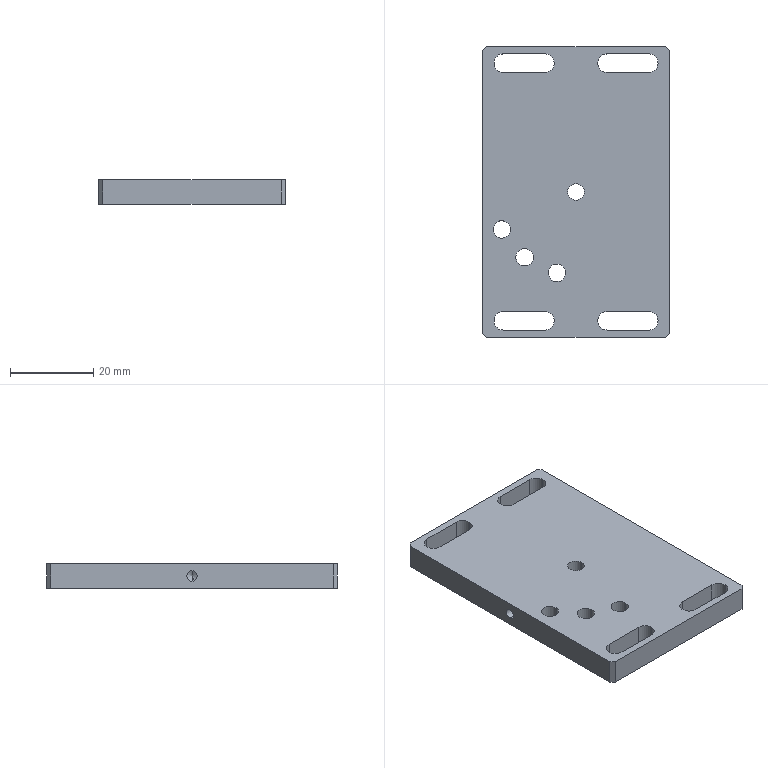Part | NX | features BREP 1 | 1 solid | 46 faces | box 45 x 70 x 6 mm | volume 16957 mm3 | cylinder 24 | plane 18 | cone 4 | commonest cylinder face diameters 4.5 x12 4.2 x6 2.5 x4 4 x2
STEP:
#1=CARTESIAN_POINT('',(2.,0.,6.));
#2=VERTEX_POINT('',#1);
#3=CARTESIAN_POINT('',(-2.,0.,6.));
#4=VERTEX_POINT('',#3);
#5=CARTESIAN_POINT('',(0.,0.,6.));
#6=DIRECTION('',(0.,0.,-1.));
#7=DIRECTION('',(-1.,0.,0.));
#8=AXIS2_PLACEMENT_3D('',#5,#6,#7);
#9=CIRCLE('',#8,2.);
#10=EDGE_CURVE('',#2,#4,#9,.T.);
#11=ORIENTED_EDGE('',*,*,#10,.F.);
#12=CARTESIAN_POINT('',(2.,0.,0.));
#13=VERTEX_POINT('',#12);
#14=CARTESIAN_POINT('',(2.,0.,0.));
#15=DIRECTION('',(0.,0.,-1.));
#16=VECTOR('',#15,1000.);
#17=LINE('',#14,#16);
#18=EDGE_CURVE('',#2,#13,#17,.T.);
#19=ORIENTED_EDGE('',*,*,#18,.T.);
#20=CARTESIAN_POINT('',(-2.,0.,0.));
#21=VERTEX_POINT('',#20);
#22=CARTESIAN_POINT('',(0.,0.,0.));
#23=DIRECTION('',(0.,0.,-1.));
#24=DIRECTION('',(-1.,0.,0.));
#25=AXIS2_PLACEMENT_3D('',#22,#23,#24);
#26=CIRCLE('',#25,2.);
#27=EDGE_CURVE('',#13,#21,#26,.T.);
#28=ORIENTED_EDGE('',*,*,#27,.T.);
#29=CARTESIAN_POINT('',(-2.,0.,0.));
#30=DIRECTION('',(0.,0.,-1.));
#31=VECTOR('',#30,1000.);
#32=LINE('',#29,#31);
#33=EDGE_CURVE('',#4,#21,#32,.T.);
#34=ORIENTED_EDGE('',*,*,#33,.F.);
#35=EDGE_LOOP('',(#11,#19,#28,#34));
#36=FACE_BOUND('',#35,.T.);
#37=CARTESIAN_POINT('',(0.,0.,0.));
#38=DIRECTION('',(0.,0.,-1.));
#39=DIRECTION('',(-1.,0.,0.));
#40=AXIS2_PLACEMENT_3D('',#37,#38,#39);
#41=CYLINDRICAL_SURFACE('',#40,2.);
#42=ADVANCED_FACE('',(#36),#41,.F.);
#43=CARTESIAN_POINT('',(-6.686,-19.467,0.));
#44=VERTEX_POINT('',#43);
#45=CARTESIAN_POINT('',(-2.486,-19.467,0.));
#46=VERTEX_POINT('',#45);
#47=CARTESIAN_POINT('',(-4.586,-19.467,0.));
#48=DIRECTION('',(0.,0.,1.));
#49=DIRECTION('',(1.,0.,0.));
#50=AXIS2_PLACEMENT_3D('',#47,#48,#49);
#51=CIRCLE('',#50,2.1);
#52=EDGE_CURVE('',#44,#46,#51,.T.);
#53=ORIENTED_EDGE('',*,*,#52,.F.);
#54=CARTESIAN_POINT('',(-6.686,-19.467,6.));
#55=VERTEX_POINT('',#54);
#56=CARTESIAN_POINT('',(-6.686,-19.467,6.));
#57=DIRECTION('',(0.,0.,1.));
#58=VECTOR('',#57,1000.);
#59=LINE('',#56,#58);
#60=EDGE_CURVE('',#55,#44,#59,.F.);
#61=ORIENTED_EDGE('',*,*,#60,.F.);
#62=CARTESIAN_POINT('',(-2.486,-19.467,6.));
#63=VERTEX_POINT('',#62);
#64=CARTESIAN_POINT('',(-4.586,-19.467,6.));
#65=DIRECTION('',(0.,0.,1.));
#66=DIRECTION('',(1.,0.,0.));
#67=AXIS2_PLACEMENT_3D('',#64,#65,#66);
#68=CIRCLE('',#67,2.1);
#69=EDGE_CURVE('',#55,#63,#68,.T.);
#70=ORIENTED_EDGE('',*,*,#69,.T.);
#71=CARTESIAN_POINT('',(-2.486,-19.467,6.));
#72=DIRECTION('',(0.,0.,1.));
#73=VECTOR('',#72,1000.);
#74=LINE('',#71,#73);
#75=EDGE_CURVE('',#63,#46,#74,.F.);
#76=ORIENTED_EDGE('',*,*,#75,.T.);
#77=EDGE_LOOP('',(#53,#61,#70,#76));
#78=FACE_BOUND('',#77,.T.);
#79=CARTESIAN_POINT('',(-4.586,-19.467,6.));
#80=DIRECTION('',(0.,0.,1.));
#81=DIRECTION('',(1.,0.,0.));
#82=AXIS2_PLACEMENT_3D('',#79,#80,#81);
#83=CYLINDRICAL_SURFACE('',#82,2.1);
#84=ADVANCED_FACE('',(#78),#83,.F.);
#85=CARTESIAN_POINT('',(-14.484,-15.705,0.));
#86=VERTEX_POINT('',#85);
#87=CARTESIAN_POINT('',(-10.284,-15.705,0.));
#88=VERTEX_POINT('',#87);
#89=CARTESIAN_POINT('',(-12.384,-15.705,0.));
#90=DIRECTION('',(0.,0.,1.));
#91=DIRECTION('',(1.,0.,0.));
#92=AXIS2_PLACEMENT_3D('',#89,#90,#91);
#93=CIRCLE('',#92,2.1);
#94=EDGE_CURVE('',#86,#88,#93,.T.);
#95=ORIENTED_EDGE('',*,*,#94,.F.);
#96=CARTESIAN_POINT('',(-14.484,-15.705,6.));
#97=VERTEX_POINT('',#96);
#98=CARTESIAN_POINT('',(-14.484,-15.705,6.));
#99=DIRECTION('',(0.,0.,1.));
#100=VECTOR('',#99,1000.);
#101=LINE('',#98,#100);
#102=EDGE_CURVE('',#97,#86,#101,.F.);
#103=ORIENTED_EDGE('',*,*,#102,.F.);
#104=CARTESIAN_POINT('',(-10.284,-15.705,6.));
#105=VERTEX_POINT('',#104);
#106=CARTESIAN_POINT('',(-12.384,-15.705,6.));
#107=DIRECTION('',(0.,0.,1.));
#108=DIRECTION('',(1.,0.,0.));
#109=AXIS2_PLACEMENT_3D('',#106,#107,#108);
#110=CIRCLE('',#109,2.1);
#111=EDGE_CURVE('',#97,#105,#110,.T.);
#112=ORIENTED_EDGE('',*,*,#111,.T.);
#113=CARTESIAN_POINT('',(-10.284,-15.705,6.));
#114=DIRECTION('',(0.,0.,1.));
#115=VECTOR('',#114,1000.);
#116=LINE('',#113,#115);
#117=EDGE_CURVE('',#105,#88,#116,.F.);
#118=ORIENTED_EDGE('',*,*,#117,.T.);
#119=EDGE_LOOP('',(#95,#103,#112,#118));
#120=FACE_BOUND('',#119,.T.);
#121=CARTESIAN_POINT('',(-12.384,-15.705,6.));
#122=DIRECTION('',(0.,0.,1.));
#123=DIRECTION('',(1.,0.,0.));
#124=AXIS2_PLACEMENT_3D('',#121,#122,#123);
#125=CYLINDRICAL_SURFACE('',#124,2.1);
#126=ADVANCED_FACE('',(#120),#125,.F.);
#127=CARTESIAN_POINT('',(-19.961,-9.,0.));
#128=VERTEX_POINT('',#127);
#129=CARTESIAN_POINT('',(-15.761,-9.,0.));
#130=VERTEX_POINT('',#129);
#131=CARTESIAN_POINT('',(-17.861,-9.,0.));
#132=DIRECTION('',(0.,0.,1.));
#133=DIRECTION('',(1.,0.,0.));
#134=AXIS2_PLACEMENT_3D('',#131,#132,#133);
#135=CIRCLE('',#134,2.1);
#136=EDGE_CURVE('',#128,#130,#135,.T.);
#137=ORIENTED_EDGE('',*,*,#136,.F.);
#138=CARTESIAN_POINT('',(-19.961,-9.,6.));
#139=VERTEX_POINT('',#138);
#140=CARTESIAN_POINT('',(-19.961,-9.,6.));
#141=DIRECTION('',(0.,0.,1.));
#142=VECTOR('',#141,1000.);
#143=LINE('',#140,#142);
#144=EDGE_CURVE('',#139,#128,#143,.F.);
#145=ORIENTED_EDGE('',*,*,#144,.F.);
#146=CARTESIAN_POINT('',(-15.761,-9.,6.));
#147=VERTEX_POINT('',#146);
#148=CARTESIAN_POINT('',(-17.861,-9.,6.));
#149=DIRECTION('',(0.,0.,1.));
#150=DIRECTION('',(1.,0.,0.));
#151=AXIS2_PLACEMENT_3D('',#148,#149,#150);
#152=CIRCLE('',#151,2.1);
#153=EDGE_CURVE('',#139,#147,#152,.T.);
#154=ORIENTED_EDGE('',*,*,#153,.T.);
#155=CARTESIAN_POINT('',(-15.761,-9.,6.));
#156=DIRECTION('',(0.,0.,1.));
#157=VECTOR('',#156,1000.);
#158=LINE('',#155,#157);
#159=EDGE_CURVE('',#147,#130,#158,.F.);
#160=ORIENTED_EDGE('',*,*,#159,.T.);
#161=EDGE_LOOP('',(#137,#145,#154,#160));
#162=FACE_BOUND('',#161,.T.);
#163=CARTESIAN_POINT('',(-17.861,-9.,6.));
#164=DIRECTION('',(0.,0.,1.));
#165=DIRECTION('',(1.,0.,0.));
#166=AXIS2_PLACEMENT_3D('',#163,#164,#165);
#167=CYLINDRICAL_SURFACE('',#166,2.1);
#168=ADVANCED_FACE('',(#162),#167,.F.);
#169=CARTESIAN_POINT('',(-8.,0.,1.75));
#170=VERTEX_POINT('',#169);
#171=CARTESIAN_POINT('',(-8.,0.,4.25));
#172=VERTEX_POINT('',#171);
#173=CARTESIAN_POINT('',(-8.,0.,3.));
#174=DIRECTION('',(-1.,0.,0.));
#175=DIRECTION('',(0.,0.,1.));
#176=AXIS2_PLACEMENT_3D('',#173,#174,#175);
#177=CIRCLE('',#176,1.25);
#178=EDGE_CURVE('',#170,#172,#177,.T.);
#179=ORIENTED_EDGE('',*,*,#178,.F.);
#180=CARTESIAN_POINT('',(-22.5,0.,1.75));
#181=VERTEX_POINT('',#180);
#182=CARTESIAN_POINT('',(-22.5,0.,1.75));
#183=DIRECTION('',(-1.,0.,0.));
#184=VECTOR('',#183,1000.);
#185=LINE('',#182,#184);
#186=EDGE_CURVE('',#181,#170,#185,.F.);
#187=ORIENTED_EDGE('',*,*,#186,.F.);
#188=CARTESIAN_POINT('',(-22.5,0.,4.25));
#189=VERTEX_POINT('',#188);
#190=CARTESIAN_POINT('',(-22.5,0.,3.));
#191=DIRECTION('',(-1.,0.,0.));
#192=DIRECTION('',(0.,0.,1.));
#193=AXIS2_PLACEMENT_3D('',#190,#191,#192);
#194=CIRCLE('',#193,1.25);
#195=EDGE_CURVE('',#181,#189,#194,.T.);
#196=ORIENTED_EDGE('',*,*,#195,.T.);
#197=CARTESIAN_POINT('',(-22.5,0.,4.25));
#198=DIRECTION('',(-1.,0.,0.));
#199=VECTOR('',#198,1000.);
#200=LINE('',#197,#199);
#201=EDGE_CURVE('',#189,#172,#200,.F.);
#202=ORIENTED_EDGE('',*,*,#201,.T.);
#203=EDGE_LOOP('',(#179,#187,#196,#202));
#204=FACE_BOUND('',#203,.T.);
#205=CARTESIAN_POINT('',(-22.5,0.,3.));
#206=DIRECTION('',(-1.,0.,0.));
#207=DIRECTION('',(0.,0.,1.));
#208=AXIS2_PLACEMENT_3D('',#205,#206,#207);
#209=CYLINDRICAL_SURFACE('',#208,1.25);
#210=ADVANCED_FACE('',(#204),#209,.F.);
#211=CARTESIAN_POINT('',(-7.249,0.,3.));
#212=VERTEX_POINT('',#211);
#213=CARTESIAN_POINT('',(-8.,0.,4.25));
#214=DIRECTION('',(-0.515,0.,0.8572));
#215=VECTOR('',#214,1000.);
#216=LINE('',#213,#215);
#217=EDGE_CURVE('',#172,#212,#216,.F.);
#218=ORIENTED_EDGE('',*,*,#217,.T.);
#219=CARTESIAN_POINT('',(-8.,0.,1.75));
#220=DIRECTION('',(-0.515,0.,-0.8572));
#221=VECTOR('',#220,1000.);
#222=LINE('',#219,#221);
#223=EDGE_CURVE('',#170,#212,#222,.F.);
#224=ORIENTED_EDGE('',*,*,#223,.F.);
#225=ORIENTED_EDGE('',*,*,#178,.T.);
#226=EDGE_LOOP('',(#218,#224,#225));
#227=FACE_BOUND('',#226,.T.);
#228=CARTESIAN_POINT('',(-8.,0.,3.));
#229=DIRECTION('',(-1.,0.,0.));
#230=DIRECTION('',(0.,0.,1.));
#231=AXIS2_PLACEMENT_3D('',#228,#229,#230);
#232=CONICAL_SURFACE('',#231,1.25,1.03);
#233=ADVANCED_FACE('',(#227),#232,.F.);
#234=CARTESIAN_POINT('',(8.,0.,4.25));
#235=VERTEX_POINT('',#234);
#236=CARTESIAN_POINT('',(8.,0.,1.75));
#237=VERTEX_POINT('',#236);
#238=CARTESIAN_POINT('',(8.,0.,3.));
#239=DIRECTION('',(1.,0.,0.));
#240=DIRECTION('',(0.,0.,-1.));
#241=AXIS2_PLACEMENT_3D('',#238,#239,#240);
#242=CIRCLE('',#241,1.25);
#243=EDGE_CURVE('',#235,#237,#242,.T.);
#244=ORIENTED_EDGE('',*,*,#243,.F.);
#245=CARTESIAN_POINT('',(22.5,0.,4.25));
#246=VERTEX_POINT('',#245);
#247=CARTESIAN_POINT('',(22.5,0.,4.25));
#248=DIRECTION('',(1.,0.,0.));
#249=VECTOR('',#248,1000.);
#250=LINE('',#247,#249);
#251=EDGE_CURVE('',#235,#246,#250,.T.);
#252=ORIENTED_EDGE('',*,*,#251,.T.);
#253=CARTESIAN_POINT('',(22.5,0.,1.75));
#254=VERTEX_POINT('',#253);
#255=CARTESIAN_POINT('',(22.5,0.,3.));
#256=DIRECTION('',(1.,0.,0.));
#257=DIRECTION('',(0.,0.,-1.));
#258=AXIS2_PLACEMENT_3D('',#255,#256,#257);
#259=CIRCLE('',#258,1.25);
#260=EDGE_CURVE('',#246,#254,#259,.T.);
#261=ORIENTED_EDGE('',*,*,#260,.T.);
#262=CARTESIAN_POINT('',(22.5,0.,1.75));
#263=DIRECTION('',(1.,0.,0.));
#264=VECTOR('',#263,1000.);
#265=LINE('',#262,#264);
#266=EDGE_CURVE('',#237,#254,#265,.T.);
#267=ORIENTED_EDGE('',*,*,#266,.F.);
#268=EDGE_LOOP('',(#244,#252,#261,#267));
#269=FACE_BOUND('',#268,.T.);
#270=CARTESIAN_POINT('',(22.5,0.,3.));
#271=DIRECTION('',(1.,0.,0.));
#272=DIRECTION('',(0.,0.,-1.));
#273=AXIS2_PLACEMENT_3D('',#270,#271,#272);
#274=CYLINDRICAL_SURFACE('',#273,1.25);
#275=ADVANCED_FACE('',(#269),#274,.F.);
#276=CARTESIAN_POINT('',(7.249,0.,3.));
#277=VERTEX_POINT('',#276);
#278=CARTESIAN_POINT('',(8.,0.,1.75));
#279=DIRECTION('',(0.515,0.,-0.8572));
#280=VECTOR('',#279,1000.);
#281=LINE('',#278,#280);
#282=EDGE_CURVE('',#277,#237,#281,.T.);
#283=ORIENTED_EDGE('',*,*,#282,.F.);
#284=CARTESIAN_POINT('',(8.,0.,4.25));
#285=DIRECTION('',(0.515,0.,0.8572));
#286=VECTOR('',#285,1000.);
#287=LINE('',#284,#286);
#288=EDGE_CURVE('',#277,#235,#287,.T.);
#289=ORIENTED_EDGE('',*,*,#288,.T.);
#290=ORIENTED_EDGE('',*,*,#243,.T.);
#291=EDGE_LOOP('',(#283,#289,#290));
#292=FACE_BOUND('',#291,.T.);
#293=CARTESIAN_POINT('',(8.,0.,3.));
#294=DIRECTION('',(1.,0.,0.));
#295=DIRECTION('',(0.,0.,-1.));
#296=AXIS2_PLACEMENT_3D('',#293,#294,#295);
#297=CONICAL_SURFACE('',#296,1.25,1.03);
#298=ADVANCED_FACE('',(#292),#297,.F.);
#299=CARTESIAN_POINT('',(17.5,-28.75,0.));
#300=VERTEX_POINT('',#299);
#301=CARTESIAN_POINT('',(19.75,-31.,0.));
#302=VERTEX_POINT('',#301);
#303=CARTESIAN_POINT('',(17.5,-31.,0.));
#304=DIRECTION('',(0.,0.,-1.));
#305=DIRECTION('',(1.,0.,0.));
#306=AXIS2_PLACEMENT_3D('',#303,#304,#305);
#307=CIRCLE('',#306,2.25);
#308=EDGE_CURVE('',#300,#302,#307,.T.);
#309=ORIENTED_EDGE('',*,*,#308,.T.);
#310=CARTESIAN_POINT('',(19.75,-31.,6.));
#311=VERTEX_POINT('',#310);
#312=CARTESIAN_POINT('',(19.75,-31.,-17.5));
#313=DIRECTION('',(0.,0.,1.));
#314=VECTOR('',#313,1000.);
#315=LINE('',#312,#314);
#316=EDGE_CURVE('',#302,#311,#315,.T.);
#317=ORIENTED_EDGE('',*,*,#316,.T.);
#318=CARTESIAN_POINT('',(17.5,-28.75,6.));
#319=VERTEX_POINT('',#318);
#320=CARTESIAN_POINT('',(17.5,-31.,6.));
#321=DIRECTION('',(0.,0.,-1.));
#322=DIRECTION('',(-1.,0.,0.));
#323=AXIS2_PLACEMENT_3D('',#320,#321,#322);
#324=CIRCLE('',#323,2.25);
#325=EDGE_CURVE('',#319,#311,#324,.T.);
#326=ORIENTED_EDGE('',*,*,#325,.F.);
#327=CARTESIAN_POINT('',(17.5,-28.75,-17.5));
#328=DIRECTION('',(0.,0.,1.));
#329=VECTOR('',#328,1000.);
#330=LINE('',#327,#329);
#331=EDGE_CURVE('',#300,#319,#330,.T.);
#332=ORIENTED_EDGE('',*,*,#331,.F.);
#333=EDGE_LOOP('',(#309,#317,#326,#332));
#334=FACE_BOUND('',#333,.T.);
#335=CARTESIAN_POINT('',(17.5,-31.,-17.5));
#336=DIRECTION('',(0.,0.,1.));
#337=DIRECTION('',(1.,0.,0.));
#338=AXIS2_PLACEMENT_3D('',#335,#336,#337);
#339=CYLINDRICAL_SURFACE('',#338,2.25);
#340=ADVANCED_FACE('',(#334),#339,.F.);
#341=CARTESIAN_POINT('',(17.5,33.25,0.));
#342=VERTEX_POINT('',#341);
#343=CARTESIAN_POINT('',(19.75,31.,0.));
#344=VERTEX_POINT('',#343);
#345=CARTESIAN_POINT('',(17.5,31.,0.));
#346=DIRECTION('',(0.,0.,-1.));
#347=DIRECTION('',(1.,0.,0.));
#348=AXIS2_PLACEMENT_3D('',#345,#346,#347);
#349=CIRCLE('',#348,2.25);
#350=EDGE_CURVE('',#342,#344,#349,.T.);
#351=ORIENTED_EDGE('',*,*,#350,.T.);
#352=CARTESIAN_POINT('',(19.75,31.,6.));
#353=VERTEX_POINT('',#352);
#354=CARTESIAN_POINT('',(19.75,31.,-17.5));
#355=DIRECTION('',(0.,0.,1.));
#356=VECTOR('',#355,1000.);
#357=LINE('',#354,#356);
#358=EDGE_CURVE('',#344,#353,#357,.T.);
#359=ORIENTED_EDGE('',*,*,#358,.T.);
#360=CARTESIAN_POINT('',(17.5,33.25,6.));
#361=VERTEX_POINT('',#360);
#362=CARTESIAN_POINT('',(17.5,31.,6.));
#363=DIRECTION('',(0.,0.,-1.));
#364=DIRECTION('',(-1.,0.,0.));
#365=AXIS2_PLACEMENT_3D('',#362,#363,#364);
#366=CIRCLE('',#365,2.25);
#367=EDGE_CURVE('',#361,#353,#366,.T.);
#368=ORIENTED_EDGE('',*,*,#367,.F.);
#369=CARTESIAN_POINT('',(17.5,33.25,-17.5));
#370=DIRECTION('',(0.,0.,1.));
#371=VECTOR('',#370,1000.);
#372=LINE('',#369,#371);
#373=EDGE_CURVE('',#342,#361,#372,.T.);
#374=ORIENTED_EDGE('',*,*,#373,.F.);
#375=EDGE_LOOP('',(#351,#359,#368,#374));
#376=FACE_BOUND('',#375,.T.);
#377=CARTESIAN_POINT('',(17.5,31.,-17.5));
#378=DIRECTION('',(0.,0.,1.));
#379=DIRECTION('',(1.,0.,0.));
#380=AXIS2_PLACEMENT_3D('',#377,#378,#379);
#381=CYLINDRICAL_SURFACE('',#380,2.25);
#382=ADVANCED_FACE('',(#376),#381,.F.);
#383=CARTESIAN_POINT('',(-5.25,-31.,0.));
#384=VERTEX_POINT('',#383);
#385=CARTESIAN_POINT('',(-7.5,-28.75,0.));
#386=VERTEX_POINT('',#385);
#387=CARTESIAN_POINT('',(-7.5,-31.,0.));
#388=DIRECTION('',(0.,0.,1.));
#389=DIRECTION('',(1.,0.,0.));
#390=AXIS2_PLACEMENT_3D('',#387,#388,#389);
#391=CIRCLE('',#390,2.25);
#392=EDGE_CURVE('',#384,#386,#391,.T.);
#393=ORIENTED_EDGE('',*,*,#392,.F.);
#394=CARTESIAN_POINT('',(-5.25,-31.,6.));
#395=VERTEX_POINT('',#394);
#396=CARTESIAN_POINT('',(-5.25,-31.,-17.5));
#397=DIRECTION('',(0.,0.,1.));
#398=VECTOR('',#397,1000.);
#399=LINE('',#396,#398);
#400=EDGE_CURVE('',#384,#395,#399,.T.);
#401=ORIENTED_EDGE('',*,*,#400,.T.);
#402=CARTESIAN_POINT('',(-7.5,-28.75,6.));
#403=VERTEX_POINT('',#402);
#404=CARTESIAN_POINT('',(-7.5,-31.,6.));
#405=DIRECTION('',(0.,0.,1.));
#406=DIRECTION('',(1.,0.,0.));
#407=AXIS2_PLACEMENT_3D('',#404,#405,#406);
#408=CIRCLE('',#407,2.25);
#409=EDGE_CURVE('',#395,#403,#408,.T.);
#410=ORIENTED_EDGE('',*,*,#409,.T.);
#411=CARTESIAN_POINT('',(-7.5,-28.75,-17.5));
#412=DIRECTION('',(0.,0.,1.));
#413=VECTOR('',#412,1000.);
#414=LINE('',#411,#413);
#415=EDGE_CURVE('',#386,#403,#414,.T.);
#416=ORIENTED_EDGE('',*,*,#415,.F.);
#417=EDGE_LOOP('',(#393,#401,#410,#416));
#418=FACE_BOUND('',#417,.T.);
#419=CARTESIAN_POINT('',(-7.5,-31.,-17.5));
#420=DIRECTION('',(0.,0.,1.));
#421=DIRECTION('',(1.,0.,0.));
#422=AXIS2_PLACEMENT_3D('',#419,#420,#421);
#423=CYLINDRICAL_SURFACE('',#422,2.25);
#424=ADVANCED_FACE('',(#418),#423,.F.);
#425=CARTESIAN_POINT('',(-5.25,31.,0.));
#426=VERTEX_POINT('',#425);
#427=CARTESIAN_POINT('',(-7.5,33.25,0.));
#428=VERTEX_POINT('',#427);
#429=CARTESIAN_POINT('',(-7.5,31.,0.));
#430=DIRECTION('',(0.,0.,1.));
#431=DIRECTION('',(1.,0.,0.));
#432=AXIS2_PLACEMENT_3D('',#429,#430,#431);
#433=CIRCLE('',#432,2.25);
#434=EDGE_CURVE('',#426,#428,#433,.T.);
#435=ORIENTED_EDGE('',*,*,#434,.F.);
#436=CARTESIAN_POINT('',(-5.25,31.,6.));
#437=VERTEX_POINT('',#436);
#438=CARTESIAN_POINT('',(-5.25,31.,-17.5));
#439=DIRECTION('',(0.,0.,1.));
#440=VECTOR('',#439,1000.);
#441=LINE('',#438,#440);
#442=EDGE_CURVE('',#426,#437,#441,.T.);
#443=ORIENTED_EDGE('',*,*,#442,.T.);
#444=CARTESIAN_POINT('',(-7.5,33.25,6.));
#445=VERTEX_POINT('',#444);
#446=CARTESIAN_POINT('',(-7.5,31.,6.));
#447=DIRECTION('',(0.,0.,1.));
#448=DIRECTION('',(1.,0.,0.));
#449=AXIS2_PLACEMENT_3D('',#446,#447,#448);
#450=CIRCLE('',#449,2.25);
#451=EDGE_CURVE('',#437,#445,#450,.T.);
#452=ORIENTED_EDGE('',*,*,#451,.T.);
#453=CARTESIAN_POINT('',(-7.5,33.25,-17.5));
#454=DIRECTION('',(0.,0.,1.));
#455=VECTOR('',#454,1000.);
#456=LINE('',#453,#455);
#457=EDGE_CURVE('',#428,#445,#456,.T.);
#458=ORIENTED_EDGE('',*,*,#457,.F.);
#459=EDGE_LOOP('',(#435,#443,#452,#458));
#460=FACE_BOUND('',#459,.T.);
#461=CARTESIAN_POINT('',(-7.5,31.,-17.5));
#462=DIRECTION('',(0.,0.,1.));
#463=DIRECTION('',(1.,0.,0.));
#464=AXIS2_PLACEMENT_3D('',#461,#462,#463);
#465=CYLINDRICAL_SURFACE('',#464,2.25);
#466=ADVANCED_FACE('',(#460),#465,.F.);
#467=CARTESIAN_POINT('',(22.5,-34.,6.));
#468=VERTEX_POINT('',#467);
#469=CARTESIAN_POINT('',(22.5,34.,6.));
#470=VERTEX_POINT('',#469);
#471=CARTESIAN_POINT('',(22.5,35.,6.));
#472=DIRECTION('',(0.,1.,0.));
#473=VECTOR('',#472,1000.);
#474=LINE('',#471,#473);
#475=EDGE_CURVE('',#468,#470,#474,.T.);
#476=ORIENTED_EDGE('',*,*,#475,.T.);
#477=CARTESIAN_POINT('',(21.5,35.,6.));
#478=VERTEX_POINT('',#477);
#479=CARTESIAN_POINT('',(28.25,28.25,6.));
#480=DIRECTION('',(-0.7071,0.7071,0.));
#481=VECTOR('',#480,1000.);
#482=LINE('',#479,#481);
#483=EDGE_CURVE('',#470,#478,#482,.T.);
#484=ORIENTED_EDGE('',*,*,#483,.T.);
#485=CARTESIAN_POINT('',(-21.5,35.,6.));
#486=VERTEX_POINT('',#485);
#487=CARTESIAN_POINT('',(-22.5,35.,6.));
#488=DIRECTION('',(-1.,0.,0.));
#489=VECTOR('',#488,1000.);
#490=LINE('',#487,#489);
#491=EDGE_CURVE('',#478,#486,#490,.T.);
#492=ORIENTED_EDGE('',*,*,#491,.T.);
#493=CARTESIAN_POINT('',(-22.5,34.,6.));
#494=VERTEX_POINT('',#493);
#495=CARTESIAN_POINT('',(-28.25,28.25,6.));
#496=DIRECTION('',(-0.7071,-0.7071,0.));
#497=VECTOR('',#496,1000.);
#498=LINE('',#495,#497);
#499=EDGE_CURVE('',#486,#494,#498,.T.);
#500=ORIENTED_EDGE('',*,*,#499,.T.);
#501=CARTESIAN_POINT('',(-22.5,-34.,6.));
#502=VERTEX_POINT('',#501);
#503=CARTESIAN_POINT('',(-22.5,35.,6.));
#504=DIRECTION('',(0.,-1.,0.));
#505=VECTOR('',#504,1000.);
#506=LINE('',#503,#505);
#507=EDGE_CURVE('',#494,#502,#506,.T.);
#508=ORIENTED_EDGE('',*,*,#507,.T.);
#509=CARTESIAN_POINT('',(-21.5,-35.,6.));
#510=VERTEX_POINT('',#509);
#511=CARTESIAN_POINT('',(-28.25,-28.25,6.));
#512=DIRECTION('',(0.7071,-0.7071,0.));
#513=VECTOR('',#512,1000.);
#514=LINE('',#511,#513);
#515=EDGE_CURVE('',#502,#510,#514,.T.);
#516=ORIENTED_EDGE('',*,*,#515,.T.);
#517=CARTESIAN_POINT('',(21.5,-35.,6.));
#518=VERTEX_POINT('',#517);
#519=CARTESIAN_POINT('',(-22.5,-35.,6.));
#520=DIRECTION('',(1.,0.,0.));
#521=VECTOR('',#520,1000.);
#522=LINE('',#519,#521);
#523=EDGE_CURVE('',#510,#518,#522,.T.);
#524=ORIENTED_EDGE('',*,*,#523,.T.);
#525=CARTESIAN_POINT('',(28.25,-28.25,6.));
#526=DIRECTION('',(0.7071,0.7071,0.));
#527=VECTOR('',#526,1000.);
#528=LINE('',#525,#527);
#529=EDGE_CURVE('',#518,#468,#528,.T.);
#530=ORIENTED_EDGE('',*,*,#529,.T.);
#531=EDGE_LOOP('',(#476,#484,#492,#500,#508,#516,#524,#530));
#532=FACE_BOUND('',#531,.T.);
#533=CARTESIAN_POINT('',(7.5,-28.75,6.));
#534=VERTEX_POINT('',#533);
#535=CARTESIAN_POINT('',(17.5,-28.75,6.));
#536=DIRECTION('',(1.,0.,0.));
#537=VECTOR('',#536,1000.);
#538=LINE('',#535,#537);
#539=EDGE_CURVE('',#534,#319,#538,.T.);
#540=ORIENTED_EDGE('',*,*,#539,.T.);
#541=ORIENTED_EDGE('',*,*,#325,.T.);
#542=CARTESIAN_POINT('',(17.5,-33.25,6.));
#543=VERTEX_POINT('',#542);
#544=CARTESIAN_POINT('',(17.5,-31.,6.));
#545=DIRECTION('',(0.,0.,-1.));
#546=DIRECTION('',(-1.,0.,0.));
#547=AXIS2_PLACEMENT_3D('',#544,#545,#546);
#548=CIRCLE('',#547,2.25);
#549=EDGE_CURVE('',#311,#543,#548,.T.);
#550=ORIENTED_EDGE('',*,*,#549,.T.);
#551=CARTESIAN_POINT('',(7.5,-33.25,6.));
#552=VERTEX_POINT('',#551);
#553=CARTESIAN_POINT('',(17.5,-33.25,6.));
#554=DIRECTION('',(-1.,0.,0.));
#555=VECTOR('',#554,1000.);
#556=LINE('',#553,#555);
#557=EDGE_CURVE('',#543,#552,#556,.T.);
#558=ORIENTED_EDGE('',*,*,#557,.T.);
#559=CARTESIAN_POINT('',(7.5,-31.,6.));
#560=DIRECTION('',(0.,0.,-1.));
#561=DIRECTION('',(-1.,0.,0.));
#562=AXIS2_PLACEMENT_3D('',#559,#560,#561);
#563=CIRCLE('',#562,2.25);
#564=EDGE_CURVE('',#552,#534,#563,.T.);
#565=ORIENTED_EDGE('',*,*,#564,.T.);
#566=EDGE_LOOP('',(#540,#541,#550,#558,#565));
#567=FACE_BOUND('',#566,.T.);
#568=CARTESIAN_POINT('',(-17.5,33.25,6.));
#569=VERTEX_POINT('',#568);
#570=CARTESIAN_POINT('',(-17.5,28.75,6.));
#571=VERTEX_POINT('',#570);
#572=CARTESIAN_POINT('',(-17.5,31.,6.));
#573=DIRECTION('',(0.,0.,1.));
#574=DIRECTION('',(1.,0.,0.));
#575=AXIS2_PLACEMENT_3D('',#572,#573,#574);
#576=CIRCLE('',#575,2.25);
#577=EDGE_CURVE('',#569,#571,#576,.T.);
#578=ORIENTED_EDGE('',*,*,#577,.F.);
#579=CARTESIAN_POINT('',(-17.5,33.25,6.));
#580=DIRECTION('',(-1.,0.,0.));
#581=VECTOR('',#580,1000.);
#582=LINE('',#579,#581);
#583=EDGE_CURVE('',#445,#569,#582,.T.);
#584=ORIENTED_EDGE('',*,*,#583,.F.);
#585=ORIENTED_EDGE('',*,*,#451,.F.);
#586=CARTESIAN_POINT('',(-7.5,28.75,6.));
#587=VERTEX_POINT('',#586);
#588=CARTESIAN_POINT('',(-7.5,31.,6.));
#589=DIRECTION('',(0.,0.,1.));
#590=DIRECTION('',(1.,0.,0.));
#591=AXIS2_PLACEMENT_3D('',#588,#589,#590);
#592=CIRCLE('',#591,2.25);
#593=EDGE_CURVE('',#587,#437,#592,.T.);
#594=ORIENTED_EDGE('',*,*,#593,.F.);
#595=CARTESIAN_POINT('',(-17.5,28.75,6.));
#596=DIRECTION('',(1.,0.,0.));
#597=VECTOR('',#596,1000.);
#598=LINE('',#595,#597);
#599=EDGE_CURVE('',#571,#587,#598,.T.);
#600=ORIENTED_EDGE('',*,*,#599,.F.);
#601=EDGE_LOOP('',(#578,#584,#585,#594,#600));
#602=FACE_BOUND('',#601,.T.);
#603=CARTESIAN_POINT('',(-17.5,-28.75,6.));
#604=VERTEX_POINT('',#603);
#605=CARTESIAN_POINT('',(-17.5,-33.25,6.));
#606=VERTEX_POINT('',#605);
#607=CARTESIAN_POINT('',(-17.5,-31.,6.));
#608=DIRECTION('',(0.,0.,1.));
#609=DIRECTION('',(1.,0.,0.));
#610=AXIS2_PLACEMENT_3D('',#607,#608,#609);
#611=CIRCLE('',#610,2.25);
#612=EDGE_CURVE('',#604,#606,#611,.T.);
#613=ORIENTED_EDGE('',*,*,#612,.F.);
#614=CARTESIAN_POINT('',(-17.5,-28.75,6.));
#615=DIRECTION('',(-1.,0.,0.));
#616=VECTOR('',#615,1000.);
#617=LINE('',#614,#616);
#618=EDGE_CURVE('',#403,#604,#617,.T.);
#619=ORIENTED_EDGE('',*,*,#618,.F.);
#620=ORIENTED_EDGE('',*,*,#409,.F.);
#621=CARTESIAN_POINT('',(-7.5,-33.25,6.));
#622=VERTEX_POINT('',#621);
#623=CARTESIAN_POINT('',(-7.5,-31.,6.));
#624=DIRECTION('',(0.,0.,1.));
#625=DIRECTION('',(1.,0.,0.));
#626=AXIS2_PLACEMENT_3D('',#623,#624,#625);
#627=CIRCLE('',#626,2.25);
#628=EDGE_CURVE('',#622,#395,#627,.T.);
#629=ORIENTED_EDGE('',*,*,#628,.F.);
#630=CARTESIAN_POINT('',(-17.5,-33.25,6.));
#631=DIRECTION('',(1.,0.,0.));
#632=VECTOR('',#631,1000.);
#633=LINE('',#630,#632);
#634=EDGE_CURVE('',#606,#622,#633,.T.);
#635=ORIENTED_EDGE('',*,*,#634,.F.);
#636=EDGE_LOOP('',(#613,#619,#620,#629,#635));
#637=FACE_BOUND('',#636,.T.);
#638=CARTESIAN_POINT('',(7.5,33.25,6.));
#639=VERTEX_POINT('',#638);
#640=CARTESIAN_POINT('',(17.5,33.25,6.));
#641=DIRECTION('',(1.,0.,0.));
#642=VECTOR('',#641,1000.);
#643=LINE('',#640,#642);
#644=EDGE_CURVE('',#639,#361,#643,.T.);
#645=ORIENTED_EDGE('',*,*,#644,.T.);
#646=ORIENTED_EDGE('',*,*,#367,.T.);
#647=CARTESIAN_POINT('',(17.5,28.75,6.));
#648=VERTEX_POINT('',#647);
#649=CARTESIAN_POINT('',(17.5,31.,6.));
#650=DIRECTION('',(0.,0.,-1.));
#651=DIRECTION('',(-1.,0.,0.));
#652=AXIS2_PLACEMENT_3D('',#649,#650,#651);
#653=CIRCLE('',#652,2.25);
#654=EDGE_CURVE('',#353,#648,#653,.T.);
#655=ORIENTED_EDGE('',*,*,#654,.T.);
#656=CARTESIAN_POINT('',(7.5,28.75,6.));
#657=VERTEX_POINT('',#656);
#658=CARTESIAN_POINT('',(17.5,28.75,6.));
#659=DIRECTION('',(-1.,0.,0.));
#660=VECTOR('',#659,1000.);
#661=LINE('',#658,#660);
#662=EDGE_CURVE('',#648,#657,#661,.T.);
#663=ORIENTED_EDGE('',*,*,#662,.T.);
#664=CARTESIAN_POINT('',(7.5,31.,6.));
#665=DIRECTION('',(0.,0.,-1.));
#666=DIRECTION('',(-1.,0.,0.));
#667=AXIS2_PLACEMENT_3D('',#664,#665,#666);
#668=CIRCLE('',#667,2.25);
#669=EDGE_CURVE('',#657,#639,#668,.T.);
#670=ORIENTED_EDGE('',*,*,#669,.T.);
#671=EDGE_LOOP('',(#645,#646,#655,#663,#670));
#672=FACE_BOUND('',#671,.T.);
#673=CARTESIAN_POINT('',(-17.861,-9.,6.));
#674=DIRECTION('',(0.,0.,1.));
#675=DIRECTION('',(1.,0.,0.));
#676=AXIS2_PLACEMENT_3D('',#673,#674,#675);
#677=CIRCLE('',#676,2.1);
#678=EDGE_CURVE('',#147,#139,#677,.T.);
#679=ORIENTED_EDGE('',*,*,#678,.F.);
#680=ORIENTED_EDGE('',*,*,#153,.F.);
#681=EDGE_LOOP('',(#679,#680));
#682=FACE_BOUND('',#681,.T.);
#683=CARTESIAN_POINT('',(-12.384,-15.705,6.));
#684=DIRECTION('',(0.,0.,1.));
#685=DIRECTION('',(1.,0.,0.));
#686=AXIS2_PLACEMENT_3D('',#683,#684,#685);
#687=CIRCLE('',#686,2.1);
#688=EDGE_CURVE('',#105,#97,#687,.T.);
#689=ORIENTED_EDGE('',*,*,#688,.F.);
#690=ORIENTED_EDGE('',*,*,#111,.F.);
#691=EDGE_LOOP('',(#689,#690));
#692=FACE_BOUND('',#691,.T.);
#693=CARTESIAN_POINT('',(-4.586,-19.467,6.));
#694=DIRECTION('',(0.,0.,1.));
#695=DIRECTION('',(1.,0.,0.));
#696=AXIS2_PLACEMENT_3D('',#693,#694,#695);
#697=CIRCLE('',#696,2.1);
#698=EDGE_CURVE('',#63,#55,#697,.T.);
#699=ORIENTED_EDGE('',*,*,#698,.F.);
#700=ORIENTED_EDGE('',*,*,#69,.F.);
#701=EDGE_LOOP('',(#699,#700));
#702=FACE_BOUND('',#701,.T.);
#703=CARTESIAN_POINT('',(0.,0.,6.));
#704=DIRECTION('',(0.,0.,-1.));
#705=DIRECTION('',(-1.,0.,0.));
#706=AXIS2_PLACEMENT_3D('',#703,#704,#705);
#707=CIRCLE('',#706,2.);
#708=EDGE_CURVE('',#4,#2,#707,.T.);
#709=ORIENTED_EDGE('',*,*,#708,.T.);
#710=ORIENTED_EDGE('',*,*,#10,.T.);
#711=EDGE_LOOP('',(#709,#710));
#712=FACE_BOUND('',#711,.T.);
#713=CARTESIAN_POINT('',(0.,0.,6.));
#714=DIRECTION('',(0.,0.,1.));
#715=DIRECTION('',(1.,0.,0.));
#716=AXIS2_PLACEMENT_3D('',#713,#714,#715);
#717=PLANE('',#716);
#718=ADVANCED_FACE('',(#532,#567,#602,#637,#672,#682,#692,#702,#712),#717,.T.);
#719=CARTESIAN_POINT('',(21.5,35.,0.));
#720=VERTEX_POINT('',#719);
#721=CARTESIAN_POINT('',(-21.5,35.,0.));
#722=VERTEX_POINT('',#721);
#723=CARTESIAN_POINT('',(-22.5,35.,0.));
#724=DIRECTION('',(-1.,0.,0.));
#725=VECTOR('',#724,1000.);
#726=LINE('',#723,#725);
#727=EDGE_CURVE('',#720,#722,#726,.T.);
#728=ORIENTED_EDGE('',*,*,#727,.F.);
#729=CARTESIAN_POINT('',(22.5,34.,0.));
#730=VERTEX_POINT('',#729);
#731=CARTESIAN_POINT('',(21.5,35.,0.));
#732=DIRECTION('',(0.7071,-0.7071,0.));
#733=VECTOR('',#732,1000.);
#734=LINE('',#731,#733);
#735=EDGE_CURVE('',#720,#730,#734,.T.);
#736=ORIENTED_EDGE('',*,*,#735,.T.);
#737=CARTESIAN_POINT('',(22.5,-34.,0.));
#738=VERTEX_POINT('',#737);
#739=CARTESIAN_POINT('',(22.5,35.,0.));
#740=DIRECTION('',(0.,1.,0.));
#741=VECTOR('',#740,1000.);
#742=LINE('',#739,#741);
#743=EDGE_CURVE('',#738,#730,#742,.T.);
#744=ORIENTED_EDGE('',*,*,#743,.F.);
#745=CARTESIAN_POINT('',(21.5,-35.,0.));
#746=VERTEX_POINT('',#745);
#747=CARTESIAN_POINT('',(22.5,-34.,0.));
#748=DIRECTION('',(-0.7071,-0.7071,0.));
#749=VECTOR('',#748,1000.);
#750=LINE('',#747,#749);
#751=EDGE_CURVE('',#738,#746,#750,.T.);
#752=ORIENTED_EDGE('',*,*,#751,.T.);
#753=CARTESIAN_POINT('',(-21.5,-35.,0.));
#754=VERTEX_POINT('',#753);
#755=CARTESIAN_POINT('',(-22.5,-35.,0.));
#756=DIRECTION('',(1.,0.,0.));
#757=VECTOR('',#756,1000.);
#758=LINE('',#755,#757);
#759=EDGE_CURVE('',#754,#746,#758,.T.);
#760=ORIENTED_EDGE('',*,*,#759,.F.);
#761=CARTESIAN_POINT('',(-22.5,-34.,0.));
#762=VERTEX_POINT('',#761);
#763=CARTESIAN_POINT('',(-21.5,-35.,0.));
#764=DIRECTION('',(-0.7071,0.7071,0.));
#765=VECTOR('',#764,1000.);
#766=LINE('',#763,#765);
#767=EDGE_CURVE('',#754,#762,#766,.T.);
#768=ORIENTED_EDGE('',*,*,#767,.T.);
#769=CARTESIAN_POINT('',(-22.5,34.,0.));
#770=VERTEX_POINT('',#769);
#771=CARTESIAN_POINT('',(-22.5,35.,0.));
#772=DIRECTION('',(0.,-1.,0.));
#773=VECTOR('',#772,1000.);
#774=LINE('',#771,#773);
#775=EDGE_CURVE('',#770,#762,#774,.T.);
#776=ORIENTED_EDGE('',*,*,#775,.F.);
#777=CARTESIAN_POINT('',(-22.5,34.,0.));
#778=DIRECTION('',(0.7071,0.7071,0.));
#779=VECTOR('',#778,1000.);
#780=LINE('',#777,#779);
#781=EDGE_CURVE('',#770,#722,#780,.T.);
#782=ORIENTED_EDGE('',*,*,#781,.T.);
#783=EDGE_LOOP('',(#728,#736,#744,#752,#760,#768,#776,#782));
#784=FACE_BOUND('',#783,.T.);
#785=ORIENTED_EDGE('',*,*,#308,.F.);
#786=CARTESIAN_POINT('',(7.5,-28.75,0.));
#787=VERTEX_POINT('',#786);
#788=CARTESIAN_POINT('',(0.,-28.75,0.));
#789=DIRECTION('',(1.,0.,0.));
#790=VECTOR('',#789,1000.);
#791=LINE('',#788,#790);
#792=EDGE_CURVE('',#787,#300,#791,.T.);
#793=ORIENTED_EDGE('',*,*,#792,.F.);
#794=CARTESIAN_POINT('',(7.5,-33.25,0.));
#795=VERTEX_POINT('',#794);
#796=CARTESIAN_POINT('',(7.5,-31.,0.));
#797=DIRECTION('',(0.,0.,-1.));
#798=DIRECTION('',(1.,0.,0.));
#799=AXIS2_PLACEMENT_3D('',#796,#797,#798);
#800=CIRCLE('',#799,2.25);
#801=EDGE_CURVE('',#795,#787,#800,.T.);
#802=ORIENTED_EDGE('',*,*,#801,.F.);
#803=CARTESIAN_POINT('',(17.5,-33.25,0.));
#804=VERTEX_POINT('',#803);
#805=CARTESIAN_POINT('',(0.,-33.25,0.));
#806=DIRECTION('',(-1.,0.,0.));
#807=VECTOR('',#806,1000.);
#808=LINE('',#805,#807);
#809=EDGE_CURVE('',#804,#795,#808,.T.);
#810=ORIENTED_EDGE('',*,*,#809,.F.);
#811=CARTESIAN_POINT('',(17.5,-31.,0.));
#812=DIRECTION('',(0.,0.,-1.));
#813=DIRECTION('',(1.,0.,0.));
#814=AXIS2_PLACEMENT_3D('',#811,#812,#813);
#815=CIRCLE('',#814,2.25);
#816=EDGE_CURVE('',#302,#804,#815,.T.);
#817=ORIENTED_EDGE('',*,*,#816,.F.);
#818=EDGE_LOOP('',(#785,#793,#802,#810,#817));
#819=FACE_BOUND('',#818,.T.);
#820=CARTESIAN_POINT('',(-17.5,33.25,0.));
#821=VERTEX_POINT('',#820);
#822=CARTESIAN_POINT('',(0.,33.25,0.));
#823=DIRECTION('',(-1.,0.,0.));
#824=VECTOR('',#823,1000.);
#825=LINE('',#822,#824);
#826=EDGE_CURVE('',#428,#821,#825,.T.);
#827=ORIENTED_EDGE('',*,*,#826,.T.);
#828=CARTESIAN_POINT('',(-17.5,28.75,0.));
#829=VERTEX_POINT('',#828);
#830=CARTESIAN_POINT('',(-17.5,31.,0.));
#831=DIRECTION('',(0.,0.,1.));
#832=DIRECTION('',(1.,0.,0.));
#833=AXIS2_PLACEMENT_3D('',#830,#831,#832);
#834=CIRCLE('',#833,2.25);
#835=EDGE_CURVE('',#821,#829,#834,.T.);
#836=ORIENTED_EDGE('',*,*,#835,.T.);
#837=CARTESIAN_POINT('',(-7.5,28.75,0.));
#838=VERTEX_POINT('',#837);
#839=CARTESIAN_POINT('',(0.,28.75,0.));
#840=DIRECTION('',(1.,0.,0.));
#841=VECTOR('',#840,1000.);
#842=LINE('',#839,#841);
#843=EDGE_CURVE('',#829,#838,#842,.T.);
#844=ORIENTED_EDGE('',*,*,#843,.T.);
#845=CARTESIAN_POINT('',(-7.5,31.,0.));
#846=DIRECTION('',(0.,0.,1.));
#847=DIRECTION('',(1.,0.,0.));
#848=AXIS2_PLACEMENT_3D('',#845,#846,#847);
#849=CIRCLE('',#848,2.25);
#850=EDGE_CURVE('',#838,#426,#849,.T.);
#851=ORIENTED_EDGE('',*,*,#850,.T.);
#852=ORIENTED_EDGE('',*,*,#434,.T.);
#853=EDGE_LOOP('',(#827,#836,#844,#851,#852));
#854=FACE_BOUND('',#853,.T.);
#855=CARTESIAN_POINT('',(-17.5,-28.75,0.));
#856=VERTEX_POINT('',#855);
#857=CARTESIAN_POINT('',(0.,-28.75,0.));
#858=DIRECTION('',(-1.,0.,0.));
#859=VECTOR('',#858,1000.);
#860=LINE('',#857,#859);
#861=EDGE_CURVE('',#386,#856,#860,.T.);
#862=ORIENTED_EDGE('',*,*,#861,.T.);
#863=CARTESIAN_POINT('',(-17.5,-33.25,0.));
#864=VERTEX_POINT('',#863);
#865=CARTESIAN_POINT('',(-17.5,-31.,0.));
#866=DIRECTION('',(0.,0.,1.));
#867=DIRECTION('',(1.,0.,0.));
#868=AXIS2_PLACEMENT_3D('',#865,#866,#867);
#869=CIRCLE('',#868,2.25);
#870=EDGE_CURVE('',#856,#864,#869,.T.);
#871=ORIENTED_EDGE('',*,*,#870,.T.);
#872=CARTESIAN_POINT('',(-7.5,-33.25,0.));
#873=VERTEX_POINT('',#872);
#874=CARTESIAN_POINT('',(0.,-33.25,0.));
#875=DIRECTION('',(1.,0.,0.));
#876=VECTOR('',#875,1000.);
#877=LINE('',#874,#876);
#878=EDGE_CURVE('',#864,#873,#877,.T.);
#879=ORIENTED_EDGE('',*,*,#878,.T.);
#880=CARTESIAN_POINT('',(-7.5,-31.,0.));
#881=DIRECTION('',(0.,0.,1.));
#882=DIRECTION('',(1.,0.,0.));
#883=AXIS2_PLACEMENT_3D('',#880,#881,#882);
#884=CIRCLE('',#883,2.25);
#885=EDGE_CURVE('',#873,#384,#884,.T.);
#886=ORIENTED_EDGE('',*,*,#885,.T.);
#887=ORIENTED_EDGE('',*,*,#392,.T.);
#888=EDGE_LOOP('',(#862,#871,#879,#886,#887));
#889=FACE_BOUND('',#888,.T.);
#890=ORIENTED_EDGE('',*,*,#350,.F.);
#891=CARTESIAN_POINT('',(7.5,33.25,0.));
#892=VERTEX_POINT('',#891);
#893=CARTESIAN_POINT('',(0.,33.25,0.));
#894=DIRECTION('',(1.,0.,0.));
#895=VECTOR('',#894,1000.);
#896=LINE('',#893,#895);
#897=EDGE_CURVE('',#892,#342,#896,.T.);
#898=ORIENTED_EDGE('',*,*,#897,.F.);
#899=CARTESIAN_POINT('',(7.5,28.75,0.));
#900=VERTEX_POINT('',#899);
#901=CARTESIAN_POINT('',(7.5,31.,0.));
#902=DIRECTION('',(0.,0.,-1.));
#903=DIRECTION('',(1.,0.,0.));
#904=AXIS2_PLACEMENT_3D('',#901,#902,#903);
#905=CIRCLE('',#904,2.25);
#906=EDGE_CURVE('',#900,#892,#905,.T.);
#907=ORIENTED_EDGE('',*,*,#906,.F.);
#908=CARTESIAN_POINT('',(17.5,28.75,0.));
#909=VERTEX_POINT('',#908);
#910=CARTESIAN_POINT('',(0.,28.75,0.));
#911=DIRECTION('',(-1.,0.,0.));
#912=VECTOR('',#911,1000.);
#913=LINE('',#910,#912);
#914=EDGE_CURVE('',#909,#900,#913,.T.);
#915=ORIENTED_EDGE('',*,*,#914,.F.);
#916=CARTESIAN_POINT('',(17.5,31.,0.));
#917=DIRECTION('',(0.,0.,-1.));
#918=DIRECTION('',(1.,0.,0.));
#919=AXIS2_PLACEMENT_3D('',#916,#917,#918);
#920=CIRCLE('',#919,2.25);
#921=EDGE_CURVE('',#344,#909,#920,.T.);
#922=ORIENTED_EDGE('',*,*,#921,.F.);
#923=EDGE_LOOP('',(#890,#898,#907,#915,#922));
#924=FACE_BOUND('',#923,.T.);
#925=CARTESIAN_POINT('',(-17.861,-9.,0.));
#926=DIRECTION('',(0.,0.,1.));
#927=DIRECTION('',(1.,0.,0.));
#928=AXIS2_PLACEMENT_3D('',#925,#926,#927);
#929=CIRCLE('',#928,2.1);
#930=EDGE_CURVE('',#130,#128,#929,.T.);
#931=ORIENTED_EDGE('',*,*,#930,.T.);
#932=ORIENTED_EDGE('',*,*,#136,.T.);
#933=EDGE_LOOP('',(#931,#932));
#934=FACE_BOUND('',#933,.T.);
#935=CARTESIAN_POINT('',(-12.384,-15.705,0.));
#936=DIRECTION('',(0.,0.,1.));
#937=DIRECTION('',(1.,0.,0.));
#938=AXIS2_PLACEMENT_3D('',#935,#936,#937);
#939=CIRCLE('',#938,2.1);
#940=EDGE_CURVE('',#88,#86,#939,.T.);
#941=ORIENTED_EDGE('',*,*,#940,.T.);
#942=ORIENTED_EDGE('',*,*,#94,.T.);
#943=EDGE_LOOP('',(#941,#942));
#944=FACE_BOUND('',#943,.T.);
#945=CARTESIAN_POINT('',(-4.586,-19.467,0.));
#946=DIRECTION('',(0.,0.,1.));
#947=DIRECTION('',(1.,0.,0.));
#948=AXIS2_PLACEMENT_3D('',#945,#946,#947);
#949=CIRCLE('',#948,2.1);
#950=EDGE_CURVE('',#46,#44,#949,.T.);
#951=ORIENTED_EDGE('',*,*,#950,.T.);
#952=ORIENTED_EDGE('',*,*,#52,.T.);
#953=EDGE_LOOP('',(#951,#952));
#954=FACE_BOUND('',#953,.T.);
#955=CARTESIAN_POINT('',(0.,0.,0.));
#956=DIRECTION('',(0.,0.,-1.));
#957=DIRECTION('',(-1.,0.,0.));
#958=AXIS2_PLACEMENT_3D('',#955,#956,#957);
#959=CIRCLE('',#958,2.);
#960=EDGE_CURVE('',#21,#13,#959,.T.);
#961=ORIENTED_EDGE('',*,*,#960,.F.);
#962=ORIENTED_EDGE('',*,*,#27,.F.);
#963=EDGE_LOOP('',(#961,#962));
#964=FACE_BOUND('',#963,.T.);
#965=CARTESIAN_POINT('',(0.,0.,0.));
#966=DIRECTION('',(0.,0.,1.));
#967=DIRECTION('',(1.,0.,0.));
#968=AXIS2_PLACEMENT_3D('',#965,#966,#967);
#969=PLANE('',#968);
#970=ADVANCED_FACE('',(#784,#819,#854,#889,#924,#934,#944,#954,#964),#969,.F.);
#971=ORIENTED_EDGE('',*,*,#743,.T.);
#972=CARTESIAN_POINT('',(22.5,34.,6.));
#973=DIRECTION('',(0.,0.,1.));
#974=VECTOR('',#973,1000.);
#975=LINE('',#972,#974);
#976=EDGE_CURVE('',#730,#470,#975,.T.);
#977=ORIENTED_EDGE('',*,*,#976,.T.);
#978=ORIENTED_EDGE('',*,*,#475,.F.);
#979=CARTESIAN_POINT('',(22.5,-34.,6.));
#980=DIRECTION('',(0.,0.,-1.));
#981=VECTOR('',#980,1000.);
#982=LINE('',#979,#981);
#983=EDGE_CURVE('',#468,#738,#982,.T.);
#984=ORIENTED_EDGE('',*,*,#983,.T.);
#985=EDGE_LOOP('',(#971,#977,#978,#984));
#986=FACE_BOUND('',#985,.T.);
#987=CARTESIAN_POINT('',(22.5,0.,3.));
#988=DIRECTION('',(1.,0.,0.));
#989=DIRECTION('',(0.,0.,-1.));
#990=AXIS2_PLACEMENT_3D('',#987,#988,#989);
#991=CIRCLE('',#990,1.25);
#992=EDGE_CURVE('',#254,#246,#991,.T.);
#993=ORIENTED_EDGE('',*,*,#992,.F.);
#994=ORIENTED_EDGE('',*,*,#260,.F.);
#995=EDGE_LOOP('',(#993,#994));
#996=FACE_BOUND('',#995,.T.);
#997=CARTESIAN_POINT('',(22.5,35.,6.));
#998=DIRECTION('',(-1.,0.,0.));
#999=DIRECTION('',(0.,1.,0.));
#1000=AXIS2_PLACEMENT_3D('',#997,#998,#999);
#1001=PLANE('',#1000);
#1002=ADVANCED_FACE('',(#986,#996),#1001,.F.);
#1003=ORIENTED_EDGE('',*,*,#491,.F.);
#1004=CARTESIAN_POINT('',(21.5,35.,6.));
#1005=DIRECTION('',(0.,0.,-1.));
#1006=VECTOR('',#1005,1000.);
#1007=LINE('',#1004,#1006);
#1008=EDGE_CURVE('',#478,#720,#1007,.T.);
#1009=ORIENTED_EDGE('',*,*,#1008,.T.);
#1010=ORIENTED_EDGE('',*,*,#727,.T.);
#1011=CARTESIAN_POINT('',(-21.5,35.,6.));
#1012=DIRECTION('',(0.,0.,1.));
#1013=VECTOR('',#1012,1000.);
#1014=LINE('',#1011,#1013);
#1015=EDGE_CURVE('',#722,#486,#1014,.T.);
#1016=ORIENTED_EDGE('',*,*,#1015,.T.);
#1017=EDGE_LOOP('',(#1003,#1009,#1010,#1016));
#1018=FACE_BOUND('',#1017,.T.);
#1019=CARTESIAN_POINT('',(-22.5,35.,6.));
#1020=DIRECTION('',(0.,-1.,0.));
#1021=DIRECTION('',(0.,0.,-1.));
#1022=AXIS2_PLACEMENT_3D('',#1019,#1020,#1021);
#1023=PLANE('',#1022);
#1024=ADVANCED_FACE('',(#1018),#1023,.F.);
#1025=ORIENTED_EDGE('',*,*,#775,.T.);
#1026=CARTESIAN_POINT('',(-22.5,-34.,6.));
#1027=DIRECTION('',(0.,0.,1.));
#1028=VECTOR('',#1027,1000.);
#1029=LINE('',#1026,#1028);
#1030=EDGE_CURVE('',#762,#502,#1029,.T.);
#1031=ORIENTED_EDGE('',*,*,#1030,.T.);
#1032=ORIENTED_EDGE('',*,*,#507,.F.);
#1033=CARTESIAN_POINT('',(-22.5,34.,6.));
#1034=DIRECTION('',(0.,0.,-1.));
#1035=VECTOR('',#1034,1000.);
#1036=LINE('',#1033,#1035);
#1037=EDGE_CURVE('',#494,#770,#1036,.T.);
#1038=ORIENTED_EDGE('',*,*,#1037,.T.);
#1039=EDGE_LOOP('',(#1025,#1031,#1032,#1038));
#1040=FACE_BOUND('',#1039,.T.);
#1041=CARTESIAN_POINT('',(-22.5,0.,3.));
#1042=DIRECTION('',(-1.,0.,0.));
#1043=DIRECTION('',(0.,0.,1.));
#1044=AXIS2_PLACEMENT_3D('',#1041,#1042,#1043);
#1045=CIRCLE('',#1044,1.25);
#1046=EDGE_CURVE('',#189,#181,#1045,.T.);
#1047=ORIENTED_EDGE('',*,*,#1046,.F.);
#1048=ORIENTED_EDGE('',*,*,#195,.F.);
#1049=EDGE_LOOP('',(#1047,#1048));
#1050=FACE_BOUND('',#1049,.T.);
#1051=CARTESIAN_POINT('',(-22.5,35.,6.));
#1052=DIRECTION('',(1.,0.,0.));
#1053=DIRECTION('',(0.,1.,0.));
#1054=AXIS2_PLACEMENT_3D('',#1051,#1052,#1053);
#1055=PLANE('',#1054);
#1056=ADVANCED_FACE('',(#1040,#1050),#1055,.F.);
#1057=ORIENTED_EDGE('',*,*,#759,.T.);
#1058=CARTESIAN_POINT('',(21.5,-35.,6.));
#1059=DIRECTION('',(0.,0.,1.));
#1060=VECTOR('',#1059,1000.);
#1061=LINE('',#1058,#1060);
#1062=EDGE_CURVE('',#746,#518,#1061,.T.);
#1063=ORIENTED_EDGE('',*,*,#1062,.T.);
#1064=ORIENTED_EDGE('',*,*,#523,.F.);
#1065=CARTESIAN_POINT('',(-21.5,-35.,6.));
#1066=DIRECTION('',(0.,0.,-1.));
#1067=VECTOR('',#1066,1000.);
#1068=LINE('',#1065,#1067);
#1069=EDGE_CURVE('',#510,#754,#1068,.T.);
#1070=ORIENTED_EDGE('',*,*,#1069,.T.);
#1071=EDGE_LOOP('',(#1057,#1063,#1064,#1070));
#1072=FACE_BOUND('',#1071,.T.);
#1073=CARTESIAN_POINT('',(-22.5,-35.,6.));
#1074=DIRECTION('',(0.,1.,0.));
#1075=DIRECTION('',(1.,0.,0.));
#1076=AXIS2_PLACEMENT_3D('',#1073,#1074,#1075);
#1077=PLANE('',#1076);
#1078=ADVANCED_FACE('',(#1072),#1077,.F.);
#1079=CARTESIAN_POINT('',(-17.5,33.25,-17.5));
#1080=DIRECTION('',(0.,0.,1.));
#1081=VECTOR('',#1080,1000.);
#1082=LINE('',#1079,#1081);
#1083=EDGE_CURVE('',#821,#569,#1082,.T.);
#1084=ORIENTED_EDGE('',*,*,#1083,.T.);
#1085=ORIENTED_EDGE('',*,*,#577,.T.);
#1086=CARTESIAN_POINT('',(-17.5,28.75,-17.5));
#1087=DIRECTION('',(0.,0.,1.));
#1088=VECTOR('',#1087,1000.);
#1089=LINE('',#1086,#1088);
#1090=EDGE_CURVE('',#829,#571,#1089,.T.);
#1091=ORIENTED_EDGE('',*,*,#1090,.F.);
#1092=ORIENTED_EDGE('',*,*,#835,.F.);
#1093=EDGE_LOOP('',(#1084,#1085,#1091,#1092));
#1094=FACE_BOUND('',#1093,.T.);
#1095=CARTESIAN_POINT('',(-17.5,31.,-17.5));
#1096=DIRECTION('',(0.,0.,1.));
#1097=DIRECTION('',(1.,0.,0.));
#1098=AXIS2_PLACEMENT_3D('',#1095,#1096,#1097);
#1099=CYLINDRICAL_SURFACE('',#1098,2.25);
#1100=ADVANCED_FACE('',(#1094),#1099,.F.);
#1101=ORIENTED_EDGE('',*,*,#457,.T.);
#1102=ORIENTED_EDGE('',*,*,#583,.T.);
#1103=ORIENTED_EDGE('',*,*,#1083,.F.);
#1104=ORIENTED_EDGE('',*,*,#826,.F.);
#1105=EDGE_LOOP('',(#1101,#1102,#1103,#1104));
#1106=FACE_BOUND('',#1105,.T.);
#1107=CARTESIAN_POINT('',(-17.5,33.25,-17.5));
#1108=DIRECTION('',(0.,1.,0.));
#1109=DIRECTION('',(1.,0.,0.));
#1110=AXIS2_PLACEMENT_3D('',#1107,#1108,#1109);
#1111=PLANE('',#1110);
#1112=ADVANCED_FACE('',(#1106),#1111,.F.);
#1113=ORIENTED_EDGE('',*,*,#442,.F.);
#1114=ORIENTED_EDGE('',*,*,#850,.F.);
#1115=CARTESIAN_POINT('',(-7.5,28.75,-17.5));
#1116=DIRECTION('',(0.,0.,1.));
#1117=VECTOR('',#1116,1000.);
#1118=LINE('',#1115,#1117);
#1119=EDGE_CURVE('',#838,#587,#1118,.T.);
#1120=ORIENTED_EDGE('',*,*,#1119,.T.);
#1121=ORIENTED_EDGE('',*,*,#593,.T.);
#1122=EDGE_LOOP('',(#1113,#1114,#1120,#1121));
#1123=FACE_BOUND('',#1122,.T.);
#1124=CARTESIAN_POINT('',(-7.5,31.,-17.5));
#1125=DIRECTION('',(0.,0.,1.));
#1126=DIRECTION('',(1.,0.,0.));
#1127=AXIS2_PLACEMENT_3D('',#1124,#1125,#1126);
#1128=CYLINDRICAL_SURFACE('',#1127,2.25);
#1129=ADVANCED_FACE('',(#1123),#1128,.F.);
#1130=ORIENTED_EDGE('',*,*,#1090,.T.);
#1131=ORIENTED_EDGE('',*,*,#599,.T.);
#1132=ORIENTED_EDGE('',*,*,#1119,.F.);
#1133=ORIENTED_EDGE('',*,*,#843,.F.);
#1134=EDGE_LOOP('',(#1130,#1131,#1132,#1133));
#1135=FACE_BOUND('',#1134,.T.);
#1136=CARTESIAN_POINT('',(-17.5,28.75,-17.5));
#1137=DIRECTION('',(0.,-1.,0.));
#1138=DIRECTION('',(0.,0.,-1.));
#1139=AXIS2_PLACEMENT_3D('',#1136,#1137,#1138);
#1140=PLANE('',#1139);
#1141=ADVANCED_FACE('',(#1135),#1140,.F.);
#1142=CARTESIAN_POINT('',(-17.5,-28.75,-17.5));
#1143=DIRECTION('',(0.,0.,1.));
#1144=VECTOR('',#1143,1000.);
#1145=LINE('',#1142,#1144);
#1146=EDGE_CURVE('',#856,#604,#1145,.T.);
#1147=ORIENTED_EDGE('',*,*,#1146,.T.);
#1148=ORIENTED_EDGE('',*,*,#612,.T.);
#1149=CARTESIAN_POINT('',(-17.5,-33.25,-17.5));
#1150=DIRECTION('',(0.,0.,1.));
#1151=VECTOR('',#1150,1000.);
#1152=LINE('',#1149,#1151);
#1153=EDGE_CURVE('',#864,#606,#1152,.T.);
#1154=ORIENTED_EDGE('',*,*,#1153,.F.);
#1155=ORIENTED_EDGE('',*,*,#870,.F.);
#1156=EDGE_LOOP('',(#1147,#1148,#1154,#1155));
#1157=FACE_BOUND('',#1156,.T.);
#1158=CARTESIAN_POINT('',(-17.5,-31.,-17.5));
#1159=DIRECTION('',(0.,0.,1.));
#1160=DIRECTION('',(1.,0.,0.));
#1161=AXIS2_PLACEMENT_3D('',#1158,#1159,#1160);
#1162=CYLINDRICAL_SURFACE('',#1161,2.25);
#1163=ADVANCED_FACE('',(#1157),#1162,.F.);
#1164=ORIENTED_EDGE('',*,*,#415,.T.);
#1165=ORIENTED_EDGE('',*,*,#618,.T.);
#1166=ORIENTED_EDGE('',*,*,#1146,.F.);
#1167=ORIENTED_EDGE('',*,*,#861,.F.);
#1168=EDGE_LOOP('',(#1164,#1165,#1166,#1167));
#1169=FACE_BOUND('',#1168,.T.);
#1170=CARTESIAN_POINT('',(-17.5,-28.75,-17.5));
#1171=DIRECTION('',(0.,1.,0.));
#1172=DIRECTION('',(1.,0.,0.));
#1173=AXIS2_PLACEMENT_3D('',#1170,#1171,#1172);
#1174=PLANE('',#1173);
#1175=ADVANCED_FACE('',(#1169),#1174,.F.);
#1176=ORIENTED_EDGE('',*,*,#400,.F.);
#1177=ORIENTED_EDGE('',*,*,#885,.F.);
#1178=CARTESIAN_POINT('',(-7.5,-33.25,-17.5));
#1179=DIRECTION('',(0.,0.,1.));
#1180=VECTOR('',#1179,1000.);
#1181=LINE('',#1178,#1180);
#1182=EDGE_CURVE('',#873,#622,#1181,.T.);
#1183=ORIENTED_EDGE('',*,*,#1182,.T.);
#1184=ORIENTED_EDGE('',*,*,#628,.T.);
#1185=EDGE_LOOP('',(#1176,#1177,#1183,#1184));
#1186=FACE_BOUND('',#1185,.T.);
#1187=CARTESIAN_POINT('',(-7.5,-31.,-17.5));
#1188=DIRECTION('',(0.,0.,1.));
#1189=DIRECTION('',(1.,0.,0.));
#1190=AXIS2_PLACEMENT_3D('',#1187,#1188,#1189);
#1191=CYLINDRICAL_SURFACE('',#1190,2.25);
#1192=ADVANCED_FACE('',(#1186),#1191,.F.);
#1193=ORIENTED_EDGE('',*,*,#1153,.T.);
#1194=ORIENTED_EDGE('',*,*,#634,.T.);
#1195=ORIENTED_EDGE('',*,*,#1182,.F.);
#1196=ORIENTED_EDGE('',*,*,#878,.F.);
#1197=EDGE_LOOP('',(#1193,#1194,#1195,#1196));
#1198=FACE_BOUND('',#1197,.T.);
#1199=CARTESIAN_POINT('',(-17.5,-33.25,-17.5));
#1200=DIRECTION('',(0.,-1.,0.));
#1201=DIRECTION('',(0.,0.,-1.));
#1202=AXIS2_PLACEMENT_3D('',#1199,#1200,#1201);
#1203=PLANE('',#1202);
#1204=ADVANCED_FACE('',(#1198),#1203,.F.);
#1205=ORIENTED_EDGE('',*,*,#483,.F.);
#1206=ORIENTED_EDGE('',*,*,#976,.F.);
#1207=ORIENTED_EDGE('',*,*,#735,.F.);
#1208=ORIENTED_EDGE('',*,*,#1008,.F.);
#1209=EDGE_LOOP('',(#1205,#1206,#1207,#1208));
#1210=FACE_BOUND('',#1209,.T.);
#1211=CARTESIAN_POINT('',(21.5,35.,6.));
#1212=DIRECTION('',(-0.7071,-0.7071,0.));
#1213=DIRECTION('',(-0.7071,0.7071,0.));
#1214=AXIS2_PLACEMENT_3D('',#1211,#1212,#1213);
#1215=PLANE('',#1214);
#1216=ADVANCED_FACE('',(#1210),#1215,.F.);
#1217=ORIENTED_EDGE('',*,*,#529,.F.);
#1218=ORIENTED_EDGE('',*,*,#1062,.F.);
#1219=ORIENTED_EDGE('',*,*,#751,.F.);
#1220=ORIENTED_EDGE('',*,*,#983,.F.);
#1221=EDGE_LOOP('',(#1217,#1218,#1219,#1220));
#1222=FACE_BOUND('',#1221,.T.);
#1223=CARTESIAN_POINT('',(22.5,-34.,6.));
#1224=DIRECTION('',(-0.7071,0.7071,0.));
#1225=DIRECTION('',(0.,0.,1.));
#1226=AXIS2_PLACEMENT_3D('',#1223,#1224,#1225);
#1227=PLANE('',#1226);
#1228=ADVANCED_FACE('',(#1222),#1227,.F.);
#1229=ORIENTED_EDGE('',*,*,#515,.F.);
#1230=ORIENTED_EDGE('',*,*,#1030,.F.);
#1231=ORIENTED_EDGE('',*,*,#767,.F.);
#1232=ORIENTED_EDGE('',*,*,#1069,.F.);
#1233=EDGE_LOOP('',(#1229,#1230,#1231,#1232));
#1234=FACE_BOUND('',#1233,.T.);
#1235=CARTESIAN_POINT('',(-21.5,-35.,6.));
#1236=DIRECTION('',(0.7071,0.7071,0.));
#1237=DIRECTION('',(0.,0.,-1.));
#1238=AXIS2_PLACEMENT_3D('',#1235,#1236,#1237);
#1239=PLANE('',#1238);
#1240=ADVANCED_FACE('',(#1234),#1239,.F.);
#1241=ORIENTED_EDGE('',*,*,#499,.F.);
#1242=ORIENTED_EDGE('',*,*,#1015,.F.);
#1243=ORIENTED_EDGE('',*,*,#781,.F.);
#1244=ORIENTED_EDGE('',*,*,#1037,.F.);
#1245=EDGE_LOOP('',(#1241,#1242,#1243,#1244));
#1246=FACE_BOUND('',#1245,.T.);
#1247=CARTESIAN_POINT('',(-22.5,34.,6.));
#1248=DIRECTION('',(0.7071,-0.7071,0.));
#1249=DIRECTION('',(0.,0.,-1.));
#1250=AXIS2_PLACEMENT_3D('',#1247,#1248,#1249);
#1251=PLANE('',#1250);
#1252=ADVANCED_FACE('',(#1246),#1251,.F.);
#1253=ORIENTED_EDGE('',*,*,#358,.F.);
#1254=ORIENTED_EDGE('',*,*,#921,.T.);
#1255=CARTESIAN_POINT('',(17.5,28.75,-17.5));
#1256=DIRECTION('',(0.,0.,1.));
#1257=VECTOR('',#1256,1000.);
#1258=LINE('',#1255,#1257);
#1259=EDGE_CURVE('',#909,#648,#1258,.T.);
#1260=ORIENTED_EDGE('',*,*,#1259,.T.);
#1261=ORIENTED_EDGE('',*,*,#654,.F.);
#1262=EDGE_LOOP('',(#1253,#1254,#1260,#1261));
#1263=FACE_BOUND('',#1262,.T.);
#1264=CARTESIAN_POINT('',(17.5,31.,-17.5));
#1265=DIRECTION('',(0.,0.,1.));
#1266=DIRECTION('',(1.,0.,0.));
#1267=AXIS2_PLACEMENT_3D('',#1264,#1265,#1266);
#1268=CYLINDRICAL_SURFACE('',#1267,2.25);
#1269=ADVANCED_FACE('',(#1263),#1268,.F.);
#1270=ORIENTED_EDGE('',*,*,#914,.T.);
#1271=CARTESIAN_POINT('',(7.5,28.75,-17.5));
#1272=DIRECTION('',(0.,0.,1.));
#1273=VECTOR('',#1272,1000.);
#1274=LINE('',#1271,#1273);
#1275=EDGE_CURVE('',#900,#657,#1274,.T.);
#1276=ORIENTED_EDGE('',*,*,#1275,.T.);
#1277=ORIENTED_EDGE('',*,*,#662,.F.);
#1278=ORIENTED_EDGE('',*,*,#1259,.F.);
#1279=EDGE_LOOP('',(#1270,#1276,#1277,#1278));
#1280=FACE_BOUND('',#1279,.T.);
#1281=CARTESIAN_POINT('',(17.5,28.75,-17.5));
#1282=DIRECTION('',(0.,1.,0.));
#1283=DIRECTION('',(1.,0.,0.));
#1284=AXIS2_PLACEMENT_3D('',#1281,#1282,#1283);
#1285=PLANE('',#1284);
#1286=ADVANCED_FACE('',(#1280),#1285,.T.);
#1287=ORIENTED_EDGE('',*,*,#906,.T.);
#1288=CARTESIAN_POINT('',(7.5,33.25,-17.5));
#1289=DIRECTION('',(0.,0.,1.));
#1290=VECTOR('',#1289,1000.);
#1291=LINE('',#1288,#1290);
#1292=EDGE_CURVE('',#892,#639,#1291,.T.);
#1293=ORIENTED_EDGE('',*,*,#1292,.T.);
#1294=ORIENTED_EDGE('',*,*,#669,.F.);
#1295=ORIENTED_EDGE('',*,*,#1275,.F.);
#1296=EDGE_LOOP('',(#1287,#1293,#1294,#1295));
#1297=FACE_BOUND('',#1296,.T.);
#1298=CARTESIAN_POINT('',(7.5,31.,-17.5));
#1299=DIRECTION('',(0.,0.,1.));
#1300=DIRECTION('',(1.,0.,0.));
#1301=AXIS2_PLACEMENT_3D('',#1298,#1299,#1300);
#1302=CYLINDRICAL_SURFACE('',#1301,2.25);
#1303=ADVANCED_FACE('',(#1297),#1302,.F.);
#1304=ORIENTED_EDGE('',*,*,#897,.T.);
#1305=ORIENTED_EDGE('',*,*,#373,.T.);
#1306=ORIENTED_EDGE('',*,*,#644,.F.);
#1307=ORIENTED_EDGE('',*,*,#1292,.F.);
#1308=EDGE_LOOP('',(#1304,#1305,#1306,#1307));
#1309=FACE_BOUND('',#1308,.T.);
#1310=CARTESIAN_POINT('',(17.5,33.25,-17.5));
#1311=DIRECTION('',(0.,-1.,0.));
#1312=DIRECTION('',(0.,0.,-1.));
#1313=AXIS2_PLACEMENT_3D('',#1310,#1311,#1312);
#1314=PLANE('',#1313);
#1315=ADVANCED_FACE('',(#1309),#1314,.T.);
#1316=ORIENTED_EDGE('',*,*,#316,.F.);
#1317=ORIENTED_EDGE('',*,*,#816,.T.);
#1318=CARTESIAN_POINT('',(17.5,-33.25,-17.5));
#1319=DIRECTION('',(0.,0.,1.));
#1320=VECTOR('',#1319,1000.);
#1321=LINE('',#1318,#1320);
#1322=EDGE_CURVE('',#804,#543,#1321,.T.);
#1323=ORIENTED_EDGE('',*,*,#1322,.T.);
#1324=ORIENTED_EDGE('',*,*,#549,.F.);
#1325=EDGE_LOOP('',(#1316,#1317,#1323,#1324));
#1326=FACE_BOUND('',#1325,.T.);
#1327=CARTESIAN_POINT('',(17.5,-31.,-17.5));
#1328=DIRECTION('',(0.,0.,1.));
#1329=DIRECTION('',(1.,0.,0.));
#1330=AXIS2_PLACEMENT_3D('',#1327,#1328,#1329);
#1331=CYLINDRICAL_SURFACE('',#1330,2.25);
#1332=ADVANCED_FACE('',(#1326),#1331,.F.);
#1333=ORIENTED_EDGE('',*,*,#809,.T.);
#1334=CARTESIAN_POINT('',(7.5,-33.25,-17.5));
#1335=DIRECTION('',(0.,0.,1.));
#1336=VECTOR('',#1335,1000.);
#1337=LINE('',#1334,#1336);
#1338=EDGE_CURVE('',#795,#552,#1337,.T.);
#1339=ORIENTED_EDGE('',*,*,#1338,.T.);
#1340=ORIENTED_EDGE('',*,*,#557,.F.);
#1341=ORIENTED_EDGE('',*,*,#1322,.F.);
#1342=EDGE_LOOP('',(#1333,#1339,#1340,#1341));
#1343=FACE_BOUND('',#1342,.T.);
#1344=CARTESIAN_POINT('',(17.5,-33.25,-17.5));
#1345=DIRECTION('',(0.,1.,0.));
#1346=DIRECTION('',(1.,0.,0.));
#1347=AXIS2_PLACEMENT_3D('',#1344,#1345,#1346);
#1348=PLANE('',#1347);
#1349=ADVANCED_FACE('',(#1343),#1348,.T.);
#1350=ORIENTED_EDGE('',*,*,#801,.T.);
#1351=CARTESIAN_POINT('',(7.5,-28.75,-17.5));
#1352=DIRECTION('',(0.,0.,1.));
#1353=VECTOR('',#1352,1000.);
#1354=LINE('',#1351,#1353);
#1355=EDGE_CURVE('',#787,#534,#1354,.T.);
#1356=ORIENTED_EDGE('',*,*,#1355,.T.);
#1357=ORIENTED_EDGE('',*,*,#564,.F.);
#1358=ORIENTED_EDGE('',*,*,#1338,.F.);
#1359=EDGE_LOOP('',(#1350,#1356,#1357,#1358));
#1360=FACE_BOUND('',#1359,.T.);
#1361=CARTESIAN_POINT('',(7.5,-31.,-17.5));
#1362=DIRECTION('',(0.,0.,1.));
#1363=DIRECTION('',(1.,0.,0.));
#1364=AXIS2_PLACEMENT_3D('',#1361,#1362,#1363);
#1365=CYLINDRICAL_SURFACE('',#1364,2.25);
#1366=ADVANCED_FACE('',(#1360),#1365,.F.);
#1367=ORIENTED_EDGE('',*,*,#792,.T.);
#1368=ORIENTED_EDGE('',*,*,#331,.T.);
#1369=ORIENTED_EDGE('',*,*,#539,.F.);
#1370=ORIENTED_EDGE('',*,*,#1355,.F.);
#1371=EDGE_LOOP('',(#1367,#1368,#1369,#1370));
#1372=FACE_BOUND('',#1371,.T.);
#1373=CARTESIAN_POINT('',(17.5,-28.75,-17.5));
#1374=DIRECTION('',(0.,-1.,0.));
#1375=DIRECTION('',(0.,0.,-1.));
#1376=AXIS2_PLACEMENT_3D('',#1373,#1374,#1375);
#1377=PLANE('',#1376);
#1378=ADVANCED_FACE('',(#1372),#1377,.T.);
#1379=ORIENTED_EDGE('',*,*,#288,.F.);
#1380=ORIENTED_EDGE('',*,*,#282,.T.);
#1381=CARTESIAN_POINT('',(8.,0.,3.));
#1382=DIRECTION('',(1.,0.,0.));
#1383=DIRECTION('',(0.,0.,-1.));
#1384=AXIS2_PLACEMENT_3D('',#1381,#1382,#1383);
#1385=CIRCLE('',#1384,1.25);
#1386=EDGE_CURVE('',#237,#235,#1385,.T.);
#1387=ORIENTED_EDGE('',*,*,#1386,.T.);
#1388=EDGE_LOOP('',(#1379,#1380,#1387));
#1389=FACE_BOUND('',#1388,.T.);
#1390=CARTESIAN_POINT('',(8.,0.,3.));
#1391=DIRECTION('',(1.,0.,0.));
#1392=DIRECTION('',(0.,0.,-1.));
#1393=AXIS2_PLACEMENT_3D('',#1390,#1391,#1392);
#1394=CONICAL_SURFACE('',#1393,1.25,1.03);
#1395=ADVANCED_FACE('',(#1389),#1394,.F.);
#1396=ORIENTED_EDGE('',*,*,#251,.F.);
#1397=ORIENTED_EDGE('',*,*,#1386,.F.);
#1398=ORIENTED_EDGE('',*,*,#266,.T.);
#1399=ORIENTED_EDGE('',*,*,#992,.T.);
#1400=EDGE_LOOP('',(#1396,#1397,#1398,#1399));
#1401=FACE_BOUND('',#1400,.T.);
#1402=CARTESIAN_POINT('',(22.5,0.,3.));
#1403=DIRECTION('',(1.,0.,0.));
#1404=DIRECTION('',(0.,0.,-1.));
#1405=AXIS2_PLACEMENT_3D('',#1402,#1403,#1404);
#1406=CYLINDRICAL_SURFACE('',#1405,1.25);
#1407=ADVANCED_FACE('',(#1401),#1406,.F.);
#1408=ORIENTED_EDGE('',*,*,#223,.T.);
#1409=ORIENTED_EDGE('',*,*,#217,.F.);
#1410=CARTESIAN_POINT('',(-8.,0.,3.));
#1411=DIRECTION('',(-1.,0.,0.));
#1412=DIRECTION('',(0.,0.,1.));
#1413=AXIS2_PLACEMENT_3D('',#1410,#1411,#1412);
#1414=CIRCLE('',#1413,1.25);
#1415=EDGE_CURVE('',#172,#170,#1414,.T.);
#1416=ORIENTED_EDGE('',*,*,#1415,.T.);
#1417=EDGE_LOOP('',(#1408,#1409,#1416));
#1418=FACE_BOUND('',#1417,.T.);
#1419=CARTESIAN_POINT('',(-8.,0.,3.));
#1420=DIRECTION('',(-1.,0.,0.));
#1421=DIRECTION('',(0.,0.,1.));
#1422=AXIS2_PLACEMENT_3D('',#1419,#1420,#1421);
#1423=CONICAL_SURFACE('',#1422,1.25,1.03);
#1424=ADVANCED_FACE('',(#1418),#1423,.F.);
#1425=ORIENTED_EDGE('',*,*,#186,.T.);
#1426=ORIENTED_EDGE('',*,*,#1415,.F.);
#1427=ORIENTED_EDGE('',*,*,#201,.F.);
#1428=ORIENTED_EDGE('',*,*,#1046,.T.);
#1429=EDGE_LOOP('',(#1425,#1426,#1427,#1428));
#1430=FACE_BOUND('',#1429,.T.);
#1431=CARTESIAN_POINT('',(-22.5,0.,3.));
#1432=DIRECTION('',(-1.,0.,0.));
#1433=DIRECTION('',(0.,0.,1.));
#1434=AXIS2_PLACEMENT_3D('',#1431,#1432,#1433);
#1435=CYLINDRICAL_SURFACE('',#1434,1.25);
#1436=ADVANCED_FACE('',(#1430),#1435,.F.);
#1437=ORIENTED_EDGE('',*,*,#144,.T.);
#1438=ORIENTED_EDGE('',*,*,#930,.F.);
#1439=ORIENTED_EDGE('',*,*,#159,.F.);
#1440=ORIENTED_EDGE('',*,*,#678,.T.);
#1441=EDGE_LOOP('',(#1437,#1438,#1439,#1440));
#1442=FACE_BOUND('',#1441,.T.);
#1443=CARTESIAN_POINT('',(-17.861,-9.,6.));
#1444=DIRECTION('',(0.,0.,1.));
#1445=DIRECTION('',(1.,0.,0.));
#1446=AXIS2_PLACEMENT_3D('',#1443,#1444,#1445);
#1447=CYLINDRICAL_SURFACE('',#1446,2.1);
#1448=ADVANCED_FACE('',(#1442),#1447,.F.);
#1449=ORIENTED_EDGE('',*,*,#102,.T.);
#1450=ORIENTED_EDGE('',*,*,#940,.F.);
#1451=ORIENTED_EDGE('',*,*,#117,.F.);
#1452=ORIENTED_EDGE('',*,*,#688,.T.);
#1453=EDGE_LOOP('',(#1449,#1450,#1451,#1452));
#1454=FACE_BOUND('',#1453,.T.);
#1455=CARTESIAN_POINT('',(-12.384,-15.705,6.));
#1456=DIRECTION('',(0.,0.,1.));
#1457=DIRECTION('',(1.,0.,0.));
#1458=AXIS2_PLACEMENT_3D('',#1455,#1456,#1457);
#1459=CYLINDRICAL_SURFACE('',#1458,2.1);
#1460=ADVANCED_FACE('',(#1454),#1459,.F.);
#1461=ORIENTED_EDGE('',*,*,#60,.T.);
#1462=ORIENTED_EDGE('',*,*,#950,.F.);
#1463=ORIENTED_EDGE('',*,*,#75,.F.);
#1464=ORIENTED_EDGE('',*,*,#698,.T.);
#1465=EDGE_LOOP('',(#1461,#1462,#1463,#1464));
#1466=FACE_BOUND('',#1465,.T.);
#1467=CARTESIAN_POINT('',(-4.586,-19.467,6.));
#1468=DIRECTION('',(0.,0.,1.));
#1469=DIRECTION('',(1.,0.,0.));
#1470=AXIS2_PLACEMENT_3D('',#1467,#1468,#1469);
#1471=CYLINDRICAL_SURFACE('',#1470,2.1);
#1472=ADVANCED_FACE('',(#1466),#1471,.F.);
#1473=ORIENTED_EDGE('',*,*,#18,.F.);
#1474=ORIENTED_EDGE('',*,*,#708,.F.);
#1475=ORIENTED_EDGE('',*,*,#33,.T.);
#1476=ORIENTED_EDGE('',*,*,#960,.T.);
#1477=EDGE_LOOP('',(#1473,#1474,#1475,#1476));
#1478=FACE_BOUND('',#1477,.T.);
#1479=CARTESIAN_POINT('',(0.,0.,0.));
#1480=DIRECTION('',(0.,0.,-1.));
#1481=DIRECTION('',(-1.,0.,0.));
#1482=AXIS2_PLACEMENT_3D('',#1479,#1480,#1481);
#1483=CYLINDRICAL_SURFACE('',#1482,2.);
#1484=ADVANCED_FACE('',(#1478),#1483,.F.);
#1485=CLOSED_SHELL('',(#42,#84,#126,#168,#210,#233,#275,#298,#340,#382,#424,#466,#718,#970,#1002,#1024,#1056,#1078,#1100,#1112,#1129,#1141,#1163,#1175,#1192,#1204,#1216,#1228,#1240,#1252,#1269,#1286,#1303,#1315,#1332,#1349,#1366,#1378,#1395,#1407,#1424,#1436,#1448,#1460,#1472,#1484));
#1486=MANIFOLD_SOLID_BREP('',#1485);
#1487=(LENGTH_UNIT()NAMED_UNIT(*)SI_UNIT(.MILLI.,.METRE.));
#1488=UNCERTAINTY_MEASURE_WITH_UNIT(LENGTH_MEASURE(0.00001),#1487,'','');
#1489=(NAMED_UNIT(*)PLANE_ANGLE_UNIT()SI_UNIT($,.RADIAN.));
#1490=(NAMED_UNIT(*)SI_UNIT($,.STERADIAN.)SOLID_ANGLE_UNIT());
#1491=(GEOMETRIC_REPRESENTATION_CONTEXT(3)GLOBAL_UNCERTAINTY_ASSIGNED_CONTEXT((#1488))GLOBAL_UNIT_ASSIGNED_CONTEXT((#1487,#1489,#1490))REPRESENTATION_CONTEXT('',''));
#1492=ADVANCED_BREP_SHAPE_REPRESENTATION('',(#1486),#1491);